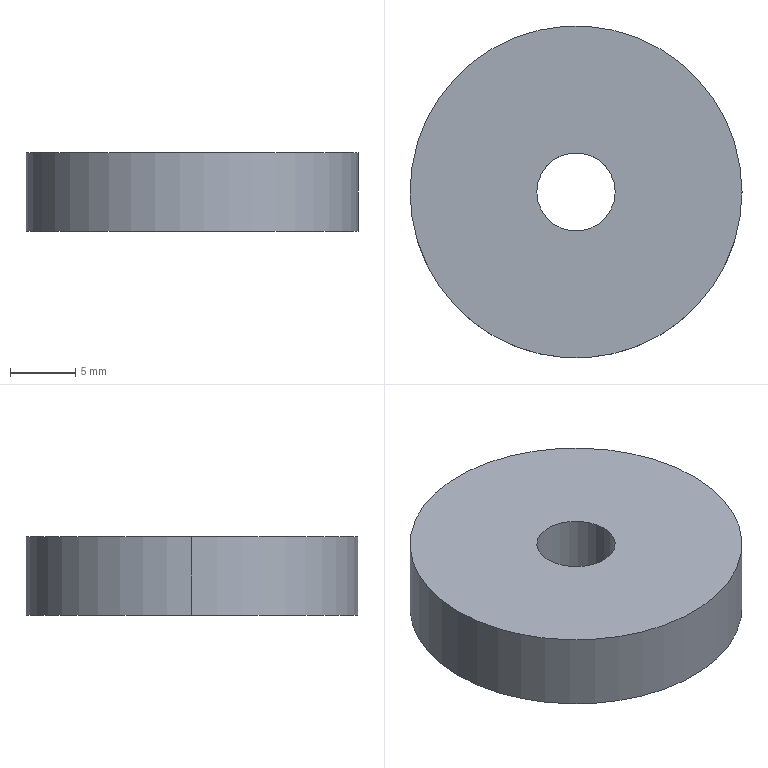Part | SolidWorks | features Extrusion 1 | 1 solid | 6 faces | box 25.4 x 25.4 x 6 mm | volume 2871 mm3 | cylinder 4 | plane 2 | commonest cylinder face diameters 6 x2 25.4 x2
STEP:
#1=CARTESIAN_POINT('',(-3.,0.,6.));
#2=VERTEX_POINT('',#1);
#3=CARTESIAN_POINT('',(3.,0.,6.));
#4=VERTEX_POINT('',#3);
#5=CARTESIAN_POINT('',(0.,0.,6.));
#6=DIRECTION('',(0.,0.,1.));
#7=DIRECTION('',(1.,0.,0.));
#8=AXIS2_PLACEMENT_3D('',#5,#6,#7);
#9=CIRCLE('',#8,3.);
#10=EDGE_CURVE('',#2,#4,#9,.T.);
#11=ORIENTED_EDGE('',*,*,#10,.T.);
#12=CARTESIAN_POINT('',(3.,0.,0.));
#13=VERTEX_POINT('',#12);
#14=CARTESIAN_POINT('',(3.,0.,6.));
#15=DIRECTION('',(0.,0.,-1.));
#16=VECTOR('',#15,1000.);
#17=LINE('',#14,#16);
#18=EDGE_CURVE('',#4,#13,#17,.T.);
#19=ORIENTED_EDGE('',*,*,#18,.T.);
#20=CARTESIAN_POINT('',(-3.,0.,0.));
#21=VERTEX_POINT('',#20);
#22=CARTESIAN_POINT('',(0.,0.,0.));
#23=DIRECTION('',(0.,0.,1.));
#24=DIRECTION('',(1.,0.,0.));
#25=AXIS2_PLACEMENT_3D('',#22,#23,#24);
#26=CIRCLE('',#25,3.);
#27=EDGE_CURVE('',#21,#13,#26,.T.);
#28=ORIENTED_EDGE('',*,*,#27,.F.);
#29=CARTESIAN_POINT('',(-3.,0.,6.));
#30=DIRECTION('',(0.,0.,-1.));
#31=VECTOR('',#30,1000.);
#32=LINE('',#29,#31);
#33=EDGE_CURVE('',#2,#21,#32,.T.);
#34=ORIENTED_EDGE('',*,*,#33,.F.);
#35=EDGE_LOOP('',(#11,#19,#28,#34));
#36=FACE_OUTER_BOUND('',#35,.T.);
#37=CARTESIAN_POINT('',(0.,0.,6.));
#38=DIRECTION('',(0.,0.,-1.));
#39=DIRECTION('',(-1.,0.,0.));
#40=AXIS2_PLACEMENT_3D('',#37,#38,#39);
#41=CYLINDRICAL_SURFACE('',#40,3.);
#42=ADVANCED_FACE('',(#36),#41,.F.);
#43=CARTESIAN_POINT('',(12.7,0.,6.));
#44=VERTEX_POINT('',#43);
#45=CARTESIAN_POINT('',(-12.7,0.,6.));
#46=VERTEX_POINT('',#45);
#47=CARTESIAN_POINT('',(0.,0.,6.));
#48=DIRECTION('',(0.,0.,1.));
#49=DIRECTION('',(1.,0.,0.));
#50=AXIS2_PLACEMENT_3D('',#47,#48,#49);
#51=CIRCLE('',#50,12.7);
#52=EDGE_CURVE('',#44,#46,#51,.T.);
#53=ORIENTED_EDGE('',*,*,#52,.F.);
#54=CARTESIAN_POINT('',(12.7,0.,0.));
#55=VERTEX_POINT('',#54);
#56=CARTESIAN_POINT('',(12.7,0.,6.));
#57=DIRECTION('',(0.,0.,-1.));
#58=VECTOR('',#57,1000.);
#59=LINE('',#56,#58);
#60=EDGE_CURVE('',#44,#55,#59,.T.);
#61=ORIENTED_EDGE('',*,*,#60,.T.);
#62=CARTESIAN_POINT('',(-12.7,0.,0.));
#63=VERTEX_POINT('',#62);
#64=CARTESIAN_POINT('',(0.,0.,0.));
#65=DIRECTION('',(0.,0.,1.));
#66=DIRECTION('',(1.,0.,0.));
#67=AXIS2_PLACEMENT_3D('',#64,#65,#66);
#68=CIRCLE('',#67,12.7);
#69=EDGE_CURVE('',#55,#63,#68,.T.);
#70=ORIENTED_EDGE('',*,*,#69,.T.);
#71=CARTESIAN_POINT('',(-12.7,0.,6.));
#72=DIRECTION('',(0.,0.,-1.));
#73=VECTOR('',#72,1000.);
#74=LINE('',#71,#73);
#75=EDGE_CURVE('',#46,#63,#74,.T.);
#76=ORIENTED_EDGE('',*,*,#75,.F.);
#77=EDGE_LOOP('',(#53,#61,#70,#76));
#78=FACE_OUTER_BOUND('',#77,.T.);
#79=CARTESIAN_POINT('',(0.,0.,6.));
#80=DIRECTION('',(0.,0.,-1.));
#81=DIRECTION('',(-1.,0.,0.));
#82=AXIS2_PLACEMENT_3D('',#79,#80,#81);
#83=CYLINDRICAL_SURFACE('',#82,12.7);
#84=ADVANCED_FACE('',(#78),#83,.T.);
#85=CARTESIAN_POINT('',(0.,0.,6.));
#86=DIRECTION('',(0.,0.,1.));
#87=DIRECTION('',(1.,0.,0.));
#88=AXIS2_PLACEMENT_3D('',#85,#86,#87);
#89=CIRCLE('',#88,12.7);
#90=EDGE_CURVE('',#46,#44,#89,.T.);
#91=ORIENTED_EDGE('',*,*,#90,.T.);
#92=ORIENTED_EDGE('',*,*,#52,.T.);
#93=EDGE_LOOP('',(#91,#92));
#94=FACE_OUTER_BOUND('',#93,.T.);
#95=ORIENTED_EDGE('',*,*,#10,.F.);
#96=CARTESIAN_POINT('',(0.,0.,6.));
#97=DIRECTION('',(0.,0.,1.));
#98=DIRECTION('',(1.,0.,0.));
#99=AXIS2_PLACEMENT_3D('',#96,#97,#98);
#100=CIRCLE('',#99,3.);
#101=EDGE_CURVE('',#4,#2,#100,.T.);
#102=ORIENTED_EDGE('',*,*,#101,.F.);
#103=EDGE_LOOP('',(#95,#102));
#104=FACE_BOUND('',#103,.T.);
#105=CARTESIAN_POINT('',(0.,0.,6.));
#106=DIRECTION('',(0.,0.,1.));
#107=DIRECTION('',(1.,0.,0.));
#108=AXIS2_PLACEMENT_3D('',#105,#106,#107);
#109=PLANE('',#108);
#110=ADVANCED_FACE('',(#94,#104),#109,.T.);
#111=CARTESIAN_POINT('',(0.,0.,0.));
#112=DIRECTION('',(0.,0.,1.));
#113=DIRECTION('',(1.,0.,0.));
#114=AXIS2_PLACEMENT_3D('',#111,#112,#113);
#115=CIRCLE('',#114,12.7);
#116=EDGE_CURVE('',#63,#55,#115,.T.);
#117=ORIENTED_EDGE('',*,*,#116,.F.);
#118=ORIENTED_EDGE('',*,*,#69,.F.);
#119=EDGE_LOOP('',(#117,#118));
#120=FACE_OUTER_BOUND('',#119,.T.);
#121=ORIENTED_EDGE('',*,*,#27,.T.);
#122=CARTESIAN_POINT('',(0.,0.,0.));
#123=DIRECTION('',(0.,0.,1.));
#124=DIRECTION('',(1.,0.,0.));
#125=AXIS2_PLACEMENT_3D('',#122,#123,#124);
#126=CIRCLE('',#125,3.);
#127=EDGE_CURVE('',#13,#21,#126,.T.);
#128=ORIENTED_EDGE('',*,*,#127,.T.);
#129=EDGE_LOOP('',(#121,#128));
#130=FACE_BOUND('',#129,.T.);
#131=CARTESIAN_POINT('',(0.,0.,0.));
#132=DIRECTION('',(0.,0.,1.));
#133=DIRECTION('',(1.,0.,0.));
#134=AXIS2_PLACEMENT_3D('',#131,#132,#133);
#135=PLANE('',#134);
#136=ADVANCED_FACE('',(#120,#130),#135,.F.);
#137=ORIENTED_EDGE('',*,*,#60,.F.);
#138=ORIENTED_EDGE('',*,*,#90,.F.);
#139=ORIENTED_EDGE('',*,*,#75,.T.);
#140=ORIENTED_EDGE('',*,*,#116,.T.);
#141=EDGE_LOOP('',(#137,#138,#139,#140));
#142=FACE_OUTER_BOUND('',#141,.T.);
#143=CARTESIAN_POINT('',(0.,0.,6.));
#144=DIRECTION('',(0.,0.,-1.));
#145=DIRECTION('',(-1.,0.,0.));
#146=AXIS2_PLACEMENT_3D('',#143,#144,#145);
#147=CYLINDRICAL_SURFACE('',#146,12.7);
#148=ADVANCED_FACE('',(#142),#147,.T.);
#149=ORIENTED_EDGE('',*,*,#18,.F.);
#150=ORIENTED_EDGE('',*,*,#101,.T.);
#151=ORIENTED_EDGE('',*,*,#33,.T.);
#152=ORIENTED_EDGE('',*,*,#127,.F.);
#153=EDGE_LOOP('',(#149,#150,#151,#152));
#154=FACE_OUTER_BOUND('',#153,.T.);
#155=CARTESIAN_POINT('',(0.,0.,6.));
#156=DIRECTION('',(0.,0.,-1.));
#157=DIRECTION('',(-1.,0.,0.));
#158=AXIS2_PLACEMENT_3D('',#155,#156,#157);
#159=CYLINDRICAL_SURFACE('',#158,3.);
#160=ADVANCED_FACE('',(#154),#159,.F.);
#161=CLOSED_SHELL('',(#42,#84,#110,#136,#148,#160));
#162=MANIFOLD_SOLID_BREP('',#161);
#163=CARTESIAN_POINT('',(0.,0.,0.));
#164=DIRECTION('',(0.,0.,1.));
#165=DIRECTION('',(1.,0.,0.));
#166=AXIS2_PLACEMENT_3D('',#163,#164,#165);
#167=(LENGTH_UNIT()NAMED_UNIT(*)SI_UNIT(.MILLI.,.METRE.));
#168=UNCERTAINTY_MEASURE_WITH_UNIT(LENGTH_MEASURE(0.00001),#167,'','');
#169=(NAMED_UNIT(*)PLANE_ANGLE_UNIT()SI_UNIT($,.RADIAN.));
#170=(NAMED_UNIT(*)SI_UNIT($,.STERADIAN.)SOLID_ANGLE_UNIT());
#171=(GEOMETRIC_REPRESENTATION_CONTEXT(3)GLOBAL_UNCERTAINTY_ASSIGNED_CONTEXT((#168))GLOBAL_UNIT_ASSIGNED_CONTEXT((#167,#169,#170))REPRESENTATION_CONTEXT('',''));
#172=ADVANCED_BREP_SHAPE_REPRESENTATION('',(#162,#166),#171);